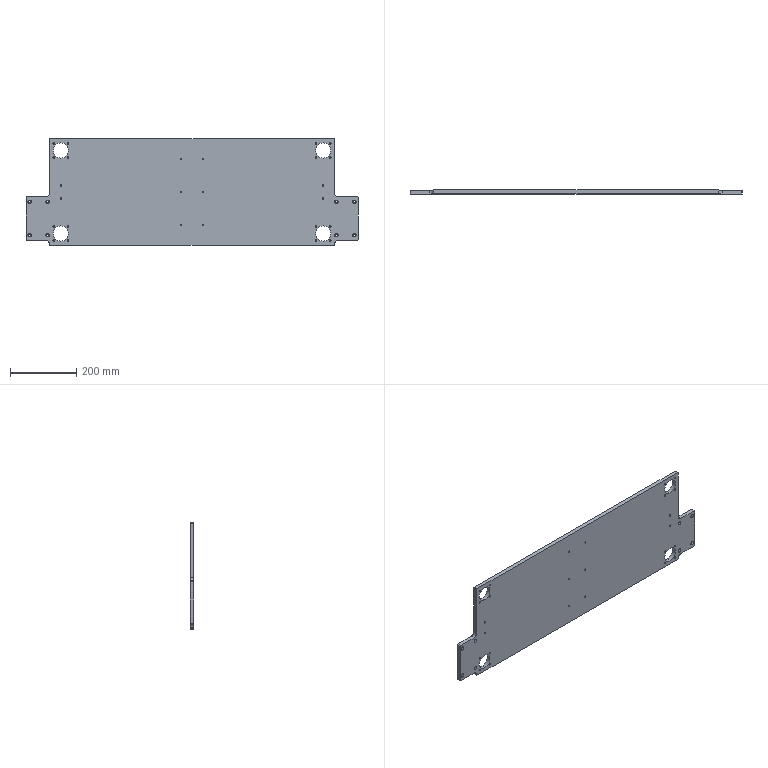Part | SolidWorks | features HoleWzd 5, Chamfer 1, Extrusion 1, ICE 1 | 1 solid | 126 faces | box 1000 x 12 x 320 mm | volume 3431289 mm3 | cylinder 96 | plane 30 | commonest cylinder face diameters 5 x40 6.6 x16 11 x16 4.2 x12 45.5 x8 20 x4